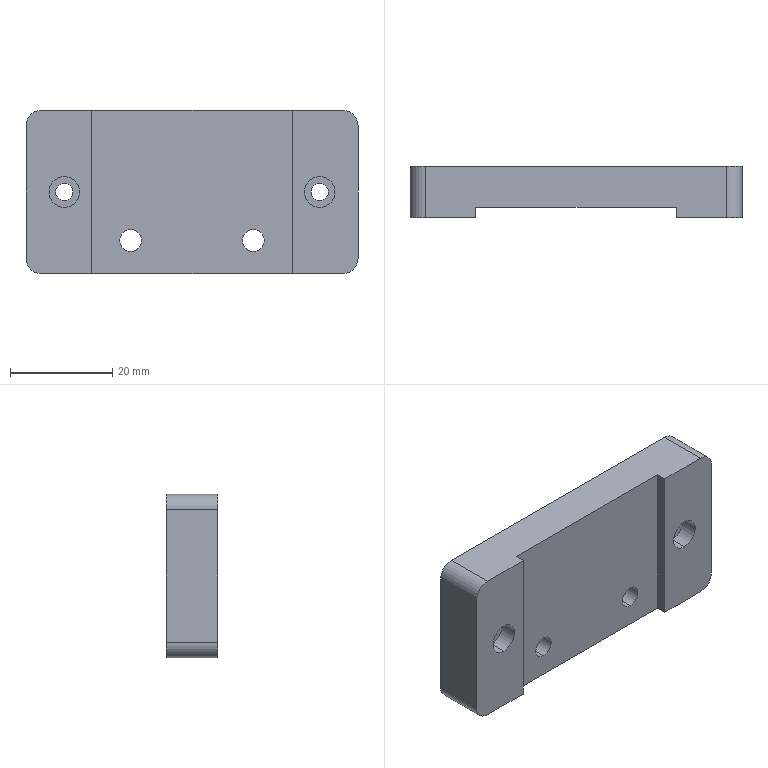Part | SolidWorks | features HoleWzd 3, ICE 3, Extrusion 1, Fillet 1 | 1 solid | 40 faces | box 65 x 10 x 32 mm | volume 16925 mm3 | cylinder 24 | plane 16 | commonest cylinder face diameters 6 x8 3.4 x4 4.3 x4 8 x4 12 x4
STEP:
#1=CARTESIAN_POINT('',(-12.,0.4,2.5));
#2=VERTEX_POINT('',#1);
#3=CARTESIAN_POINT('',(-12.,0.4,10.5));
#4=VERTEX_POINT('',#3);
#5=CARTESIAN_POINT('',(-12.,0.4,6.5));
#6=DIRECTION('',(0.,1.,0.));
#7=DIRECTION('',(0.,0.,1.));
#8=AXIS2_PLACEMENT_3D('',#5,#6,#7);
#9=CIRCLE('',#8,4.);
#10=EDGE_CURVE('',#2,#4,#9,.T.);
#11=ORIENTED_EDGE('',*,*,#10,.F.);
#12=CARTESIAN_POINT('',(-12.,5.,2.5));
#13=VERTEX_POINT('',#12);
#14=CARTESIAN_POINT('',(-12.,5.,2.5));
#15=DIRECTION('',(0.,1.,0.));
#16=VECTOR('',#15,1000.);
#17=LINE('',#14,#16);
#18=EDGE_CURVE('',#2,#13,#17,.T.);
#19=ORIENTED_EDGE('',*,*,#18,.T.);
#20=CARTESIAN_POINT('',(-12.,5.,10.5));
#21=VERTEX_POINT('',#20);
#22=CARTESIAN_POINT('',(-12.,5.,6.5));
#23=DIRECTION('',(0.,1.,0.));
#24=DIRECTION('',(0.,0.,1.));
#25=AXIS2_PLACEMENT_3D('',#22,#23,#24);
#26=CIRCLE('',#25,4.);
#27=EDGE_CURVE('',#13,#21,#26,.T.);
#28=ORIENTED_EDGE('',*,*,#27,.T.);
#29=CARTESIAN_POINT('',(-12.,5.,10.5));
#30=DIRECTION('',(0.,1.,0.));
#31=VECTOR('',#30,1000.);
#32=LINE('',#29,#31);
#33=EDGE_CURVE('',#4,#21,#32,.T.);
#34=ORIENTED_EDGE('',*,*,#33,.F.);
#35=EDGE_LOOP('',(#11,#19,#28,#34));
#36=FACE_OUTER_BOUND('',#35,.T.);
#37=CARTESIAN_POINT('',(-12.,5.,6.5));
#38=DIRECTION('',(0.,1.,0.));
#39=DIRECTION('',(0.,0.,1.));
#40=AXIS2_PLACEMENT_3D('',#37,#38,#39);
#41=CYLINDRICAL_SURFACE('',#40,4.);
#42=ADVANCED_FACE('',(#36),#41,.F.);
#43=CARTESIAN_POINT('',(12.,0.4,2.5));
#44=VERTEX_POINT('',#43);
#45=CARTESIAN_POINT('',(12.,0.4,10.5));
#46=VERTEX_POINT('',#45);
#47=CARTESIAN_POINT('',(12.,0.4,6.5));
#48=DIRECTION('',(0.,1.,0.));
#49=DIRECTION('',(0.,0.,1.));
#50=AXIS2_PLACEMENT_3D('',#47,#48,#49);
#51=CIRCLE('',#50,4.);
#52=EDGE_CURVE('',#44,#46,#51,.T.);
#53=ORIENTED_EDGE('',*,*,#52,.F.);
#54=CARTESIAN_POINT('',(12.,5.,2.5));
#55=VERTEX_POINT('',#54);
#56=CARTESIAN_POINT('',(12.,5.,2.5));
#57=DIRECTION('',(0.,1.,0.));
#58=VECTOR('',#57,1000.);
#59=LINE('',#56,#58);
#60=EDGE_CURVE('',#44,#55,#59,.T.);
#61=ORIENTED_EDGE('',*,*,#60,.T.);
#62=CARTESIAN_POINT('',(12.,5.,10.5));
#63=VERTEX_POINT('',#62);
#64=CARTESIAN_POINT('',(12.,5.,6.5));
#65=DIRECTION('',(0.,1.,0.));
#66=DIRECTION('',(0.,0.,1.));
#67=AXIS2_PLACEMENT_3D('',#64,#65,#66);
#68=CIRCLE('',#67,4.);
#69=EDGE_CURVE('',#55,#63,#68,.T.);
#70=ORIENTED_EDGE('',*,*,#69,.T.);
#71=CARTESIAN_POINT('',(12.,5.,10.5));
#72=DIRECTION('',(0.,1.,0.));
#73=VECTOR('',#72,1000.);
#74=LINE('',#71,#73);
#75=EDGE_CURVE('',#46,#63,#74,.T.);
#76=ORIENTED_EDGE('',*,*,#75,.F.);
#77=EDGE_LOOP('',(#53,#61,#70,#76));
#78=FACE_OUTER_BOUND('',#77,.T.);
#79=CARTESIAN_POINT('',(12.,5.,6.5));
#80=DIRECTION('',(0.,1.,0.));
#81=DIRECTION('',(0.,0.,1.));
#82=AXIS2_PLACEMENT_3D('',#79,#80,#81);
#83=CYLINDRICAL_SURFACE('',#82,4.);
#84=ADVANCED_FACE('',(#78),#83,.F.);
#85=CARTESIAN_POINT('',(25.,-1.6,19.));
#86=VERTEX_POINT('',#85);
#87=CARTESIAN_POINT('',(25.,-1.6,13.));
#88=VERTEX_POINT('',#87);
#89=CARTESIAN_POINT('',(25.,-1.6,16.));
#90=DIRECTION('',(0.,-1.,0.));
#91=DIRECTION('',(0.,0.,-1.));
#92=AXIS2_PLACEMENT_3D('',#89,#90,#91);
#93=CIRCLE('',#92,3.);
#94=EDGE_CURVE('',#86,#88,#93,.T.);
#95=ORIENTED_EDGE('',*,*,#94,.F.);
#96=CARTESIAN_POINT('',(25.,-5.,19.));
#97=VERTEX_POINT('',#96);
#98=CARTESIAN_POINT('',(25.,-5.,19.));
#99=DIRECTION('',(0.,-1.,0.));
#100=VECTOR('',#99,1000.);
#101=LINE('',#98,#100);
#102=EDGE_CURVE('',#86,#97,#101,.T.);
#103=ORIENTED_EDGE('',*,*,#102,.T.);
#104=CARTESIAN_POINT('',(25.,-5.,13.));
#105=VERTEX_POINT('',#104);
#106=CARTESIAN_POINT('',(25.,-5.,16.));
#107=DIRECTION('',(0.,-1.,0.));
#108=DIRECTION('',(0.,0.,-1.));
#109=AXIS2_PLACEMENT_3D('',#106,#107,#108);
#110=CIRCLE('',#109,3.);
#111=EDGE_CURVE('',#97,#105,#110,.T.);
#112=ORIENTED_EDGE('',*,*,#111,.T.);
#113=CARTESIAN_POINT('',(25.,-5.,13.));
#114=DIRECTION('',(0.,-1.,0.));
#115=VECTOR('',#114,1000.);
#116=LINE('',#113,#115);
#117=EDGE_CURVE('',#88,#105,#116,.T.);
#118=ORIENTED_EDGE('',*,*,#117,.F.);
#119=EDGE_LOOP('',(#95,#103,#112,#118));
#120=FACE_OUTER_BOUND('',#119,.T.);
#121=CARTESIAN_POINT('',(25.,-5.,16.));
#122=DIRECTION('',(0.,-1.,0.));
#123=DIRECTION('',(0.,0.,-1.));
#124=AXIS2_PLACEMENT_3D('',#121,#122,#123);
#125=CYLINDRICAL_SURFACE('',#124,3.);
#126=ADVANCED_FACE('',(#120),#125,.F.);
#127=CARTESIAN_POINT('',(25.,3.,17.7));
#128=VERTEX_POINT('',#127);
#129=CARTESIAN_POINT('',(25.,3.,14.3));
#130=VERTEX_POINT('',#129);
#131=CARTESIAN_POINT('',(25.,3.,16.));
#132=DIRECTION('',(0.,-1.,0.));
#133=DIRECTION('',(0.,0.,-1.));
#134=AXIS2_PLACEMENT_3D('',#131,#132,#133);
#135=CIRCLE('',#134,1.7);
#136=EDGE_CURVE('',#128,#130,#135,.T.);
#137=ORIENTED_EDGE('',*,*,#136,.F.);
#138=CARTESIAN_POINT('',(25.,-1.6,17.7));
#139=VERTEX_POINT('',#138);
#140=CARTESIAN_POINT('',(25.,-5.,17.7));
#141=DIRECTION('',(0.,-1.,0.));
#142=VECTOR('',#141,1000.);
#143=LINE('',#140,#142);
#144=EDGE_CURVE('',#128,#139,#143,.T.);
#145=ORIENTED_EDGE('',*,*,#144,.T.);
#146=CARTESIAN_POINT('',(25.,-1.6,14.3));
#147=VERTEX_POINT('',#146);
#148=CARTESIAN_POINT('',(25.,-1.6,16.));
#149=DIRECTION('',(0.,-1.,0.));
#150=DIRECTION('',(0.,0.,-1.));
#151=AXIS2_PLACEMENT_3D('',#148,#149,#150);
#152=CIRCLE('',#151,1.7);
#153=EDGE_CURVE('',#139,#147,#152,.T.);
#154=ORIENTED_EDGE('',*,*,#153,.T.);
#155=CARTESIAN_POINT('',(25.,-5.,14.3));
#156=DIRECTION('',(0.,-1.,0.));
#157=VECTOR('',#156,1000.);
#158=LINE('',#155,#157);
#159=EDGE_CURVE('',#130,#147,#158,.T.);
#160=ORIENTED_EDGE('',*,*,#159,.F.);
#161=EDGE_LOOP('',(#137,#145,#154,#160));
#162=FACE_OUTER_BOUND('',#161,.T.);
#163=CARTESIAN_POINT('',(25.,-5.,16.));
#164=DIRECTION('',(0.,-1.,0.));
#165=DIRECTION('',(0.,0.,-1.));
#166=AXIS2_PLACEMENT_3D('',#163,#164,#165);
#167=CYLINDRICAL_SURFACE('',#166,1.7);
#168=ADVANCED_FACE('',(#162),#167,.F.);
#169=CARTESIAN_POINT('',(-25.,-1.6,19.));
#170=VERTEX_POINT('',#169);
#171=CARTESIAN_POINT('',(-25.,-1.6,13.));
#172=VERTEX_POINT('',#171);
#173=CARTESIAN_POINT('',(-25.,-1.6,16.));
#174=DIRECTION('',(0.,-1.,0.));
#175=DIRECTION('',(0.,0.,-1.));
#176=AXIS2_PLACEMENT_3D('',#173,#174,#175);
#177=CIRCLE('',#176,3.);
#178=EDGE_CURVE('',#170,#172,#177,.T.);
#179=ORIENTED_EDGE('',*,*,#178,.F.);
#180=CARTESIAN_POINT('',(-25.,-5.,19.));
#181=VERTEX_POINT('',#180);
#182=CARTESIAN_POINT('',(-25.,-5.,19.));
#183=DIRECTION('',(0.,-1.,0.));
#184=VECTOR('',#183,1000.);
#185=LINE('',#182,#184);
#186=EDGE_CURVE('',#170,#181,#185,.T.);
#187=ORIENTED_EDGE('',*,*,#186,.T.);
#188=CARTESIAN_POINT('',(-25.,-5.,13.));
#189=VERTEX_POINT('',#188);
#190=CARTESIAN_POINT('',(-25.,-5.,16.));
#191=DIRECTION('',(0.,-1.,0.));
#192=DIRECTION('',(0.,0.,-1.));
#193=AXIS2_PLACEMENT_3D('',#190,#191,#192);
#194=CIRCLE('',#193,3.);
#195=EDGE_CURVE('',#181,#189,#194,.T.);
#196=ORIENTED_EDGE('',*,*,#195,.T.);
#197=CARTESIAN_POINT('',(-25.,-5.,13.));
#198=DIRECTION('',(0.,-1.,0.));
#199=VECTOR('',#198,1000.);
#200=LINE('',#197,#199);
#201=EDGE_CURVE('',#172,#189,#200,.T.);
#202=ORIENTED_EDGE('',*,*,#201,.F.);
#203=EDGE_LOOP('',(#179,#187,#196,#202));
#204=FACE_OUTER_BOUND('',#203,.T.);
#205=CARTESIAN_POINT('',(-25.,-5.,16.));
#206=DIRECTION('',(0.,-1.,0.));
#207=DIRECTION('',(0.,0.,-1.));
#208=AXIS2_PLACEMENT_3D('',#205,#206,#207);
#209=CYLINDRICAL_SURFACE('',#208,3.);
#210=ADVANCED_FACE('',(#204),#209,.F.);
#211=CARTESIAN_POINT('',(-25.,3.,14.3));
#212=VERTEX_POINT('',#211);
#213=CARTESIAN_POINT('',(-25.,3.,17.7));
#214=VERTEX_POINT('',#213);
#215=CARTESIAN_POINT('',(-25.,3.,16.));
#216=DIRECTION('',(0.,1.,0.));
#217=DIRECTION('',(0.,0.,1.));
#218=AXIS2_PLACEMENT_3D('',#215,#216,#217);
#219=CIRCLE('',#218,1.7);
#220=EDGE_CURVE('',#212,#214,#219,.T.);
#221=ORIENTED_EDGE('',*,*,#220,.T.);
#222=CARTESIAN_POINT('',(-25.,-1.6,17.7));
#223=VERTEX_POINT('',#222);
#224=CARTESIAN_POINT('',(-25.,-5.,17.7));
#225=DIRECTION('',(0.,-1.,0.));
#226=VECTOR('',#225,1000.);
#227=LINE('',#224,#226);
#228=EDGE_CURVE('',#214,#223,#227,.T.);
#229=ORIENTED_EDGE('',*,*,#228,.T.);
#230=CARTESIAN_POINT('',(-25.,-1.6,14.3));
#231=VERTEX_POINT('',#230);
#232=CARTESIAN_POINT('',(-25.,-1.6,16.));
#233=DIRECTION('',(0.,-1.,0.));
#234=DIRECTION('',(0.,0.,-1.));
#235=AXIS2_PLACEMENT_3D('',#232,#233,#234);
#236=CIRCLE('',#235,1.7);
#237=EDGE_CURVE('',#223,#231,#236,.T.);
#238=ORIENTED_EDGE('',*,*,#237,.T.);
#239=CARTESIAN_POINT('',(-25.,-5.,14.3));
#240=DIRECTION('',(0.,-1.,0.));
#241=VECTOR('',#240,1000.);
#242=LINE('',#239,#241);
#243=EDGE_CURVE('',#212,#231,#242,.T.);
#244=ORIENTED_EDGE('',*,*,#243,.F.);
#245=EDGE_LOOP('',(#221,#229,#238,#244));
#246=FACE_OUTER_BOUND('',#245,.T.);
#247=CARTESIAN_POINT('',(-25.,-5.,16.));
#248=DIRECTION('',(0.,-1.,0.));
#249=DIRECTION('',(0.,0.,-1.));
#250=AXIS2_PLACEMENT_3D('',#247,#248,#249);
#251=CYLINDRICAL_SURFACE('',#250,1.7);
#252=ADVANCED_FACE('',(#246),#251,.F.);
#253=CARTESIAN_POINT('',(25.,3.,10.));
#254=VERTEX_POINT('',#253);
#255=CARTESIAN_POINT('',(25.,3.,22.));
#256=VERTEX_POINT('',#255);
#257=CARTESIAN_POINT('',(25.,3.,16.));
#258=DIRECTION('',(0.,1.,0.));
#259=DIRECTION('',(0.,0.,-1.));
#260=AXIS2_PLACEMENT_3D('',#257,#258,#259);
#261=CIRCLE('',#260,6.);
#262=EDGE_CURVE('',#254,#256,#261,.T.);
#263=ORIENTED_EDGE('',*,*,#262,.F.);
#264=CARTESIAN_POINT('',(25.,5.,10.));
#265=VERTEX_POINT('',#264);
#266=CARTESIAN_POINT('',(25.,3.,10.));
#267=DIRECTION('',(0.,1.,0.));
#268=VECTOR('',#267,1000.);
#269=LINE('',#266,#268);
#270=EDGE_CURVE('',#254,#265,#269,.T.);
#271=ORIENTED_EDGE('',*,*,#270,.T.);
#272=CARTESIAN_POINT('',(25.,5.,22.));
#273=VERTEX_POINT('',#272);
#274=CARTESIAN_POINT('',(25.,5.,16.));
#275=DIRECTION('',(0.,1.,0.));
#276=DIRECTION('',(0.,0.,-1.));
#277=AXIS2_PLACEMENT_3D('',#274,#275,#276);
#278=CIRCLE('',#277,6.);
#279=EDGE_CURVE('',#265,#273,#278,.T.);
#280=ORIENTED_EDGE('',*,*,#279,.T.);
#281=CARTESIAN_POINT('',(25.,3.,22.));
#282=DIRECTION('',(0.,1.,0.));
#283=VECTOR('',#282,1000.);
#284=LINE('',#281,#283);
#285=EDGE_CURVE('',#256,#273,#284,.T.);
#286=ORIENTED_EDGE('',*,*,#285,.F.);
#287=EDGE_LOOP('',(#263,#271,#280,#286));
#288=FACE_OUTER_BOUND('',#287,.T.);
#289=CARTESIAN_POINT('',(25.,3.,16.));
#290=DIRECTION('',(0.,1.,0.));
#291=DIRECTION('',(0.,0.,1.));
#292=AXIS2_PLACEMENT_3D('',#289,#290,#291);
#293=CYLINDRICAL_SURFACE('',#292,6.);
#294=ADVANCED_FACE('',(#288),#293,.F.);
#295=CARTESIAN_POINT('',(-25.,3.,10.));
#296=VERTEX_POINT('',#295);
#297=CARTESIAN_POINT('',(-25.,3.,22.));
#298=VERTEX_POINT('',#297);
#299=CARTESIAN_POINT('',(-25.,3.,16.));
#300=DIRECTION('',(0.,1.,0.));
#301=DIRECTION('',(0.,0.,1.));
#302=AXIS2_PLACEMENT_3D('',#299,#300,#301);
#303=CIRCLE('',#302,6.);
#304=EDGE_CURVE('',#296,#298,#303,.T.);
#305=ORIENTED_EDGE('',*,*,#304,.F.);
#306=CARTESIAN_POINT('',(-25.,5.,10.));
#307=VERTEX_POINT('',#306);
#308=CARTESIAN_POINT('',(-25.,3.,10.));
#309=DIRECTION('',(0.,1.,0.));
#310=VECTOR('',#309,1000.);
#311=LINE('',#308,#310);
#312=EDGE_CURVE('',#296,#307,#311,.T.);
#313=ORIENTED_EDGE('',*,*,#312,.T.);
#314=CARTESIAN_POINT('',(-25.,5.,22.));
#315=VERTEX_POINT('',#314);
#316=CARTESIAN_POINT('',(-25.,5.,16.));
#317=DIRECTION('',(0.,1.,0.));
#318=DIRECTION('',(0.,0.,1.));
#319=AXIS2_PLACEMENT_3D('',#316,#317,#318);
#320=CIRCLE('',#319,6.);
#321=EDGE_CURVE('',#307,#315,#320,.T.);
#322=ORIENTED_EDGE('',*,*,#321,.T.);
#323=CARTESIAN_POINT('',(-25.,3.,22.));
#324=DIRECTION('',(0.,1.,0.));
#325=VECTOR('',#324,1000.);
#326=LINE('',#323,#325);
#327=EDGE_CURVE('',#298,#315,#326,.T.);
#328=ORIENTED_EDGE('',*,*,#327,.F.);
#329=EDGE_LOOP('',(#305,#313,#322,#328));
#330=FACE_OUTER_BOUND('',#329,.T.);
#331=CARTESIAN_POINT('',(-25.,3.,16.));
#332=DIRECTION('',(0.,1.,0.));
#333=DIRECTION('',(0.,0.,1.));
#334=AXIS2_PLACEMENT_3D('',#331,#332,#333);
#335=CYLINDRICAL_SURFACE('',#334,6.);
#336=ADVANCED_FACE('',(#330),#335,.F.);
#337=CARTESIAN_POINT('',(-12.,0.4,4.35));
#338=VERTEX_POINT('',#337);
#339=CARTESIAN_POINT('',(-12.,0.4,8.65));
#340=VERTEX_POINT('',#339);
#341=CARTESIAN_POINT('',(-12.,0.4,6.5));
#342=DIRECTION('',(0.,1.,0.));
#343=DIRECTION('',(0.,0.,1.));
#344=AXIS2_PLACEMENT_3D('',#341,#342,#343);
#345=CIRCLE('',#344,2.15);
#346=EDGE_CURVE('',#338,#340,#345,.T.);
#347=ORIENTED_EDGE('',*,*,#346,.T.);
#348=CARTESIAN_POINT('',(-12.,-3.,8.65));
#349=VERTEX_POINT('',#348);
#350=CARTESIAN_POINT('',(-12.,-5.,8.65));
#351=DIRECTION('',(0.,-1.,0.));
#352=VECTOR('',#351,1000.);
#353=LINE('',#350,#352);
#354=EDGE_CURVE('',#340,#349,#353,.T.);
#355=ORIENTED_EDGE('',*,*,#354,.T.);
#356=CARTESIAN_POINT('',(-12.,-3.,4.35));
#357=VERTEX_POINT('',#356);
#358=CARTESIAN_POINT('',(-12.,-3.,6.5));
#359=DIRECTION('',(0.,-1.,0.));
#360=DIRECTION('',(0.,0.,1.));
#361=AXIS2_PLACEMENT_3D('',#358,#359,#360);
#362=CIRCLE('',#361,2.15);
#363=EDGE_CURVE('',#349,#357,#362,.T.);
#364=ORIENTED_EDGE('',*,*,#363,.T.);
#365=CARTESIAN_POINT('',(-12.,-5.,4.35));
#366=DIRECTION('',(0.,-1.,0.));
#367=VECTOR('',#366,1000.);
#368=LINE('',#365,#367);
#369=EDGE_CURVE('',#338,#357,#368,.T.);
#370=ORIENTED_EDGE('',*,*,#369,.F.);
#371=EDGE_LOOP('',(#347,#355,#364,#370));
#372=FACE_OUTER_BOUND('',#371,.T.);
#373=CARTESIAN_POINT('',(-12.,-5.,6.5));
#374=DIRECTION('',(0.,-1.,0.));
#375=DIRECTION('',(0.,0.,-1.));
#376=AXIS2_PLACEMENT_3D('',#373,#374,#375);
#377=CYLINDRICAL_SURFACE('',#376,2.15);
#378=ADVANCED_FACE('',(#372),#377,.F.);
#379=CARTESIAN_POINT('',(12.,0.4,4.35));
#380=VERTEX_POINT('',#379);
#381=CARTESIAN_POINT('',(12.,0.4,8.65));
#382=VERTEX_POINT('',#381);
#383=CARTESIAN_POINT('',(12.,0.4,6.5));
#384=DIRECTION('',(0.,1.,0.));
#385=DIRECTION('',(0.,0.,1.));
#386=AXIS2_PLACEMENT_3D('',#383,#384,#385);
#387=CIRCLE('',#386,2.15);
#388=EDGE_CURVE('',#380,#382,#387,.T.);
#389=ORIENTED_EDGE('',*,*,#388,.T.);
#390=CARTESIAN_POINT('',(12.,-3.,8.65));
#391=VERTEX_POINT('',#390);
#392=CARTESIAN_POINT('',(12.,-5.,8.65));
#393=DIRECTION('',(0.,-1.,0.));
#394=VECTOR('',#393,1000.);
#395=LINE('',#392,#394);
#396=EDGE_CURVE('',#382,#391,#395,.T.);
#397=ORIENTED_EDGE('',*,*,#396,.T.);
#398=CARTESIAN_POINT('',(12.,-3.,4.35));
#399=VERTEX_POINT('',#398);
#400=CARTESIAN_POINT('',(12.,-3.,6.5));
#401=DIRECTION('',(0.,-1.,0.));
#402=DIRECTION('',(0.,0.,1.));
#403=AXIS2_PLACEMENT_3D('',#400,#401,#402);
#404=CIRCLE('',#403,2.15);
#405=EDGE_CURVE('',#391,#399,#404,.T.);
#406=ORIENTED_EDGE('',*,*,#405,.T.);
#407=CARTESIAN_POINT('',(12.,-5.,4.35));
#408=DIRECTION('',(0.,-1.,0.));
#409=VECTOR('',#408,1000.);
#410=LINE('',#407,#409);
#411=EDGE_CURVE('',#380,#399,#410,.T.);
#412=ORIENTED_EDGE('',*,*,#411,.F.);
#413=EDGE_LOOP('',(#389,#397,#406,#412));
#414=FACE_OUTER_BOUND('',#413,.T.);
#415=CARTESIAN_POINT('',(12.,-5.,6.5));
#416=DIRECTION('',(0.,-1.,0.));
#417=DIRECTION('',(0.,0.,-1.));
#418=AXIS2_PLACEMENT_3D('',#415,#416,#417);
#419=CYLINDRICAL_SURFACE('',#418,2.15);
#420=ADVANCED_FACE('',(#414),#419,.F.);
#421=CARTESIAN_POINT('',(25.,-5.,16.));
#422=DIRECTION('',(0.,-1.,0.));
#423=DIRECTION('',(0.,0.,-1.));
#424=AXIS2_PLACEMENT_3D('',#421,#422,#423);
#425=CIRCLE('',#424,3.);
#426=EDGE_CURVE('',#105,#97,#425,.T.);
#427=ORIENTED_EDGE('',*,*,#426,.F.);
#428=ORIENTED_EDGE('',*,*,#111,.F.);
#429=EDGE_LOOP('',(#427,#428));
#430=FACE_BOUND('',#429,.T.);
#431=CARTESIAN_POINT('',(19.6,-5.,32.));
#432=VERTEX_POINT('',#431);
#433=CARTESIAN_POINT('',(29.5,-5.,32.));
#434=VERTEX_POINT('',#433);
#435=CARTESIAN_POINT('',(-32.5,-5.,32.));
#436=DIRECTION('',(1.,0.,0.));
#437=VECTOR('',#436,1000.);
#438=LINE('',#435,#437);
#439=EDGE_CURVE('',#432,#434,#438,.T.);
#440=ORIENTED_EDGE('',*,*,#439,.F.);
#441=CARTESIAN_POINT('',(19.6,-5.,0.));
#442=VERTEX_POINT('',#441);
#443=CARTESIAN_POINT('',(19.6,-5.,-36.442));
#444=DIRECTION('',(0.,0.,1.));
#445=VECTOR('',#444,1000.);
#446=LINE('',#443,#445);
#447=EDGE_CURVE('',#442,#432,#446,.T.);
#448=ORIENTED_EDGE('',*,*,#447,.F.);
#449=CARTESIAN_POINT('',(29.5,-5.,0.));
#450=VERTEX_POINT('',#449);
#451=CARTESIAN_POINT('',(-32.5,-5.,0.));
#452=DIRECTION('',(1.,0.,0.));
#453=VECTOR('',#452,1000.);
#454=LINE('',#451,#453);
#455=EDGE_CURVE('',#442,#450,#454,.T.);
#456=ORIENTED_EDGE('',*,*,#455,.T.);
#457=CARTESIAN_POINT('',(32.5,-5.,3.));
#458=VERTEX_POINT('',#457);
#459=CARTESIAN_POINT('',(29.5,-5.,3.));
#460=DIRECTION('',(0.,-1.,0.));
#461=DIRECTION('',(0.,0.,1.));
#462=AXIS2_PLACEMENT_3D('',#459,#460,#461);
#463=CIRCLE('',#462,3.);
#464=EDGE_CURVE('',#450,#458,#463,.T.);
#465=ORIENTED_EDGE('',*,*,#464,.T.);
#466=CARTESIAN_POINT('',(32.5,-5.,29.));
#467=VERTEX_POINT('',#466);
#468=CARTESIAN_POINT('',(32.5,-5.,32.));
#469=DIRECTION('',(0.,0.,-1.));
#470=VECTOR('',#469,1000.);
#471=LINE('',#468,#470);
#472=EDGE_CURVE('',#467,#458,#471,.T.);
#473=ORIENTED_EDGE('',*,*,#472,.F.);
#474=CARTESIAN_POINT('',(29.5,-5.,29.));
#475=DIRECTION('',(0.,-1.,0.));
#476=DIRECTION('',(0.,0.,1.));
#477=AXIS2_PLACEMENT_3D('',#474,#475,#476);
#478=CIRCLE('',#477,3.);
#479=EDGE_CURVE('',#467,#434,#478,.T.);
#480=ORIENTED_EDGE('',*,*,#479,.T.);
#481=EDGE_LOOP('',(#440,#448,#456,#465,#473,#480));
#482=FACE_OUTER_BOUND('',#481,.T.);
#483=CARTESIAN_POINT('',(-32.5,-5.,32.));
#484=DIRECTION('',(0.,1.,0.));
#485=DIRECTION('',(0.,0.,1.));
#486=AXIS2_PLACEMENT_3D('',#483,#484,#485);
#487=PLANE('',#486);
#488=ADVANCED_FACE('',(#430,#482),#487,.F.);
#489=CARTESIAN_POINT('',(-12.,5.,6.5));
#490=DIRECTION('',(0.,1.,0.));
#491=DIRECTION('',(0.,0.,1.));
#492=AXIS2_PLACEMENT_3D('',#489,#490,#491);
#493=CIRCLE('',#492,4.);
#494=EDGE_CURVE('',#21,#13,#493,.T.);
#495=ORIENTED_EDGE('',*,*,#494,.F.);
#496=ORIENTED_EDGE('',*,*,#27,.F.);
#497=EDGE_LOOP('',(#495,#496));
#498=FACE_BOUND('',#497,.T.);
#499=CARTESIAN_POINT('',(29.5,5.,0.));
#500=VERTEX_POINT('',#499);
#501=CARTESIAN_POINT('',(-29.5,5.,0.));
#502=VERTEX_POINT('',#501);
#503=CARTESIAN_POINT('',(-32.5,5.,0.));
#504=DIRECTION('',(-1.,0.,0.));
#505=VECTOR('',#504,1000.);
#506=LINE('',#503,#505);
#507=EDGE_CURVE('',#500,#502,#506,.T.);
#508=ORIENTED_EDGE('',*,*,#507,.T.);
#509=CARTESIAN_POINT('',(-32.5,5.,3.));
#510=VERTEX_POINT('',#509);
#511=CARTESIAN_POINT('',(-29.5,5.,3.));
#512=DIRECTION('',(0.,1.,0.));
#513=DIRECTION('',(0.,0.,-1.));
#514=AXIS2_PLACEMENT_3D('',#511,#512,#513);
#515=CIRCLE('',#514,3.);
#516=EDGE_CURVE('',#502,#510,#515,.T.);
#517=ORIENTED_EDGE('',*,*,#516,.T.);
#518=CARTESIAN_POINT('',(-32.5,5.,29.));
#519=VERTEX_POINT('',#518);
#520=CARTESIAN_POINT('',(-32.5,5.,32.));
#521=DIRECTION('',(0.,0.,-1.));
#522=VECTOR('',#521,1000.);
#523=LINE('',#520,#522);
#524=EDGE_CURVE('',#519,#510,#523,.T.);
#525=ORIENTED_EDGE('',*,*,#524,.F.);
#526=CARTESIAN_POINT('',(-29.5,5.,32.));
#527=VERTEX_POINT('',#526);
#528=CARTESIAN_POINT('',(-29.5,5.,29.));
#529=DIRECTION('',(0.,1.,0.));
#530=DIRECTION('',(0.,0.,-1.));
#531=AXIS2_PLACEMENT_3D('',#528,#529,#530);
#532=CIRCLE('',#531,3.);
#533=EDGE_CURVE('',#519,#527,#532,.T.);
#534=ORIENTED_EDGE('',*,*,#533,.T.);
#535=CARTESIAN_POINT('',(29.5,5.,32.));
#536=VERTEX_POINT('',#535);
#537=CARTESIAN_POINT('',(-32.5,5.,32.));
#538=DIRECTION('',(-1.,0.,0.));
#539=VECTOR('',#538,1000.);
#540=LINE('',#537,#539);
#541=EDGE_CURVE('',#536,#527,#540,.T.);
#542=ORIENTED_EDGE('',*,*,#541,.F.);
#543=CARTESIAN_POINT('',(32.5,5.,29.));
#544=VERTEX_POINT('',#543);
#545=CARTESIAN_POINT('',(29.5,5.,29.));
#546=DIRECTION('',(0.,1.,0.));
#547=DIRECTION('',(0.,0.,-1.));
#548=AXIS2_PLACEMENT_3D('',#545,#546,#547);
#549=CIRCLE('',#548,3.);
#550=EDGE_CURVE('',#536,#544,#549,.T.);
#551=ORIENTED_EDGE('',*,*,#550,.T.);
#552=CARTESIAN_POINT('',(32.5,5.,3.));
#553=VERTEX_POINT('',#552);
#554=CARTESIAN_POINT('',(32.5,5.,32.));
#555=DIRECTION('',(0.,0.,-1.));
#556=VECTOR('',#555,1000.);
#557=LINE('',#554,#556);
#558=EDGE_CURVE('',#544,#553,#557,.T.);
#559=ORIENTED_EDGE('',*,*,#558,.T.);
#560=CARTESIAN_POINT('',(29.5,5.,3.));
#561=DIRECTION('',(0.,1.,0.));
#562=DIRECTION('',(0.,0.,-1.));
#563=AXIS2_PLACEMENT_3D('',#560,#561,#562);
#564=CIRCLE('',#563,3.);
#565=EDGE_CURVE('',#553,#500,#564,.T.);
#566=ORIENTED_EDGE('',*,*,#565,.T.);
#567=EDGE_LOOP('',(#508,#517,#525,#534,#542,#551,#559,#566));
#568=FACE_OUTER_BOUND('',#567,.T.);
#569=CARTESIAN_POINT('',(-25.,5.,16.));
#570=DIRECTION('',(0.,1.,0.));
#571=DIRECTION('',(0.,0.,1.));
#572=AXIS2_PLACEMENT_3D('',#569,#570,#571);
#573=CIRCLE('',#572,6.);
#574=EDGE_CURVE('',#315,#307,#573,.T.);
#575=ORIENTED_EDGE('',*,*,#574,.F.);
#576=ORIENTED_EDGE('',*,*,#321,.F.);
#577=EDGE_LOOP('',(#575,#576));
#578=FACE_BOUND('',#577,.T.);
#579=CARTESIAN_POINT('',(25.,5.,16.));
#580=DIRECTION('',(0.,1.,0.));
#581=DIRECTION('',(0.,0.,-1.));
#582=AXIS2_PLACEMENT_3D('',#579,#580,#581);
#583=CIRCLE('',#582,6.);
#584=EDGE_CURVE('',#273,#265,#583,.T.);
#585=ORIENTED_EDGE('',*,*,#584,.F.);
#586=ORIENTED_EDGE('',*,*,#279,.F.);
#587=EDGE_LOOP('',(#585,#586));
#588=FACE_BOUND('',#587,.T.);
#589=CARTESIAN_POINT('',(12.,5.,6.5));
#590=DIRECTION('',(0.,1.,0.));
#591=DIRECTION('',(0.,0.,1.));
#592=AXIS2_PLACEMENT_3D('',#589,#590,#591);
#593=CIRCLE('',#592,4.);
#594=EDGE_CURVE('',#63,#55,#593,.T.);
#595=ORIENTED_EDGE('',*,*,#594,.F.);
#596=ORIENTED_EDGE('',*,*,#69,.F.);
#597=EDGE_LOOP('',(#595,#596));
#598=FACE_BOUND('',#597,.T.);
#599=CARTESIAN_POINT('',(-32.5,5.,32.));
#600=DIRECTION('',(0.,-1.,0.));
#601=DIRECTION('',(0.,0.,-1.));
#602=AXIS2_PLACEMENT_3D('',#599,#600,#601);
#603=PLANE('',#602);
#604=ADVANCED_FACE('',(#498,#568,#578,#588,#598),#603,.F.);
#605=ORIENTED_EDGE('',*,*,#472,.T.);
#606=CARTESIAN_POINT('',(32.5,5.,3.));
#607=DIRECTION('',(0.,1.,0.));
#608=VECTOR('',#607,1000.);
#609=LINE('',#606,#608);
#610=EDGE_CURVE('',#458,#553,#609,.T.);
#611=ORIENTED_EDGE('',*,*,#610,.T.);
#612=ORIENTED_EDGE('',*,*,#558,.F.);
#613=CARTESIAN_POINT('',(32.5,-5.,29.));
#614=DIRECTION('',(0.,-1.,0.));
#615=VECTOR('',#614,1000.);
#616=LINE('',#613,#615);
#617=EDGE_CURVE('',#544,#467,#616,.T.);
#618=ORIENTED_EDGE('',*,*,#617,.T.);
#619=EDGE_LOOP('',(#605,#611,#612,#618));
#620=FACE_OUTER_BOUND('',#619,.T.);
#621=CARTESIAN_POINT('',(32.5,5.,32.));
#622=DIRECTION('',(-1.,0.,0.));
#623=DIRECTION('',(0.,0.,1.));
#624=AXIS2_PLACEMENT_3D('',#621,#622,#623);
#625=PLANE('',#624);
#626=ADVANCED_FACE('',(#620),#625,.F.);
#627=ORIENTED_EDGE('',*,*,#524,.T.);
#628=CARTESIAN_POINT('',(-32.5,-5.,3.));
#629=VERTEX_POINT('',#628);
#630=CARTESIAN_POINT('',(-32.5,5.,3.));
#631=DIRECTION('',(0.,-1.,0.));
#632=VECTOR('',#631,1000.);
#633=LINE('',#630,#632);
#634=EDGE_CURVE('',#510,#629,#633,.T.);
#635=ORIENTED_EDGE('',*,*,#634,.T.);
#636=CARTESIAN_POINT('',(-32.5,-5.,29.));
#637=VERTEX_POINT('',#636);
#638=CARTESIAN_POINT('',(-32.5,-5.,32.));
#639=DIRECTION('',(0.,0.,-1.));
#640=VECTOR('',#639,1000.);
#641=LINE('',#638,#640);
#642=EDGE_CURVE('',#637,#629,#641,.T.);
#643=ORIENTED_EDGE('',*,*,#642,.F.);
#644=CARTESIAN_POINT('',(-32.5,5.,29.));
#645=DIRECTION('',(0.,1.,0.));
#646=VECTOR('',#645,1000.);
#647=LINE('',#644,#646);
#648=EDGE_CURVE('',#637,#519,#647,.T.);
#649=ORIENTED_EDGE('',*,*,#648,.T.);
#650=EDGE_LOOP('',(#627,#635,#643,#649));
#651=FACE_OUTER_BOUND('',#650,.T.);
#652=CARTESIAN_POINT('',(-32.5,5.,32.));
#653=DIRECTION('',(1.,0.,0.));
#654=DIRECTION('',(0.,0.,-1.));
#655=AXIS2_PLACEMENT_3D('',#652,#653,#654);
#656=PLANE('',#655);
#657=ADVANCED_FACE('',(#651),#656,.F.);
#658=CARTESIAN_POINT('',(-25.,-5.,16.));
#659=DIRECTION('',(0.,-1.,0.));
#660=DIRECTION('',(0.,0.,-1.));
#661=AXIS2_PLACEMENT_3D('',#658,#659,#660);
#662=CIRCLE('',#661,3.);
#663=EDGE_CURVE('',#189,#181,#662,.T.);
#664=ORIENTED_EDGE('',*,*,#663,.F.);
#665=ORIENTED_EDGE('',*,*,#195,.F.);
#666=EDGE_LOOP('',(#664,#665));
#667=FACE_BOUND('',#666,.T.);
#668=CARTESIAN_POINT('',(-29.5,-5.,0.));
#669=VERTEX_POINT('',#668);
#670=CARTESIAN_POINT('',(-19.6,-5.,0.));
#671=VERTEX_POINT('',#670);
#672=CARTESIAN_POINT('',(-32.5,-5.,0.));
#673=DIRECTION('',(1.,0.,0.));
#674=VECTOR('',#673,1000.);
#675=LINE('',#672,#674);
#676=EDGE_CURVE('',#669,#671,#675,.T.);
#677=ORIENTED_EDGE('',*,*,#676,.T.);
#678=CARTESIAN_POINT('',(-19.6,-5.,32.));
#679=VERTEX_POINT('',#678);
#680=CARTESIAN_POINT('',(-19.6,-5.,-36.442));
#681=DIRECTION('',(0.,0.,-1.));
#682=VECTOR('',#681,1000.);
#683=LINE('',#680,#682);
#684=EDGE_CURVE('',#679,#671,#683,.T.);
#685=ORIENTED_EDGE('',*,*,#684,.F.);
#686=CARTESIAN_POINT('',(-29.5,-5.,32.));
#687=VERTEX_POINT('',#686);
#688=CARTESIAN_POINT('',(-32.5,-5.,32.));
#689=DIRECTION('',(1.,0.,0.));
#690=VECTOR('',#689,1000.);
#691=LINE('',#688,#690);
#692=EDGE_CURVE('',#687,#679,#691,.T.);
#693=ORIENTED_EDGE('',*,*,#692,.F.);
#694=CARTESIAN_POINT('',(-29.5,-5.,29.));
#695=DIRECTION('',(0.,-1.,0.));
#696=DIRECTION('',(0.,0.,1.));
#697=AXIS2_PLACEMENT_3D('',#694,#695,#696);
#698=CIRCLE('',#697,3.);
#699=EDGE_CURVE('',#687,#637,#698,.T.);
#700=ORIENTED_EDGE('',*,*,#699,.T.);
#701=ORIENTED_EDGE('',*,*,#642,.T.);
#702=CARTESIAN_POINT('',(-29.5,-5.,3.));
#703=DIRECTION('',(0.,-1.,0.));
#704=DIRECTION('',(0.,0.,1.));
#705=AXIS2_PLACEMENT_3D('',#702,#703,#704);
#706=CIRCLE('',#705,3.);
#707=EDGE_CURVE('',#629,#669,#706,.T.);
#708=ORIENTED_EDGE('',*,*,#707,.T.);
#709=EDGE_LOOP('',(#677,#685,#693,#700,#701,#708));
#710=FACE_OUTER_BOUND('',#709,.T.);
#711=CARTESIAN_POINT('',(-32.5,-5.,32.));
#712=DIRECTION('',(0.,1.,0.));
#713=DIRECTION('',(0.,0.,1.));
#714=AXIS2_PLACEMENT_3D('',#711,#712,#713);
#715=PLANE('',#714);
#716=ADVANCED_FACE('',(#667,#710),#715,.F.);
#717=CARTESIAN_POINT('',(19.6,-3.,32.));
#718=VERTEX_POINT('',#717);
#719=CARTESIAN_POINT('',(19.6,0.,32.));
#720=DIRECTION('',(0.,1.,0.));
#721=VECTOR('',#720,1000.);
#722=LINE('',#719,#721);
#723=EDGE_CURVE('',#432,#718,#722,.T.);
#724=ORIENTED_EDGE('',*,*,#723,.F.);
#725=ORIENTED_EDGE('',*,*,#439,.T.);
#726=CARTESIAN_POINT('',(29.5,5.,32.));
#727=DIRECTION('',(0.,1.,0.));
#728=VECTOR('',#727,1000.);
#729=LINE('',#726,#728);
#730=EDGE_CURVE('',#434,#536,#729,.T.);
#731=ORIENTED_EDGE('',*,*,#730,.T.);
#732=ORIENTED_EDGE('',*,*,#541,.T.);
#733=CARTESIAN_POINT('',(-29.5,-5.,32.));
#734=DIRECTION('',(0.,-1.,0.));
#735=VECTOR('',#734,1000.);
#736=LINE('',#733,#735);
#737=EDGE_CURVE('',#527,#687,#736,.T.);
#738=ORIENTED_EDGE('',*,*,#737,.T.);
#739=ORIENTED_EDGE('',*,*,#692,.T.);
#740=CARTESIAN_POINT('',(-19.6,-3.,32.));
#741=VERTEX_POINT('',#740);
#742=CARTESIAN_POINT('',(-19.6,0.,32.));
#743=DIRECTION('',(0.,-1.,0.));
#744=VECTOR('',#743,1000.);
#745=LINE('',#742,#744);
#746=EDGE_CURVE('',#741,#679,#745,.T.);
#747=ORIENTED_EDGE('',*,*,#746,.F.);
#748=CARTESIAN_POINT('',(0.,-3.,32.));
#749=DIRECTION('',(-1.,0.,0.));
#750=VECTOR('',#749,1000.);
#751=LINE('',#748,#750);
#752=EDGE_CURVE('',#718,#741,#751,.T.);
#753=ORIENTED_EDGE('',*,*,#752,.F.);
#754=EDGE_LOOP('',(#724,#725,#731,#732,#738,#739,#747,#753));
#755=FACE_OUTER_BOUND('',#754,.T.);
#756=CARTESIAN_POINT('',(0.,0.,32.));
#757=DIRECTION('',(0.,0.,1.));
#758=DIRECTION('',(1.,0.,0.));
#759=AXIS2_PLACEMENT_3D('',#756,#757,#758);
#760=PLANE('',#759);
#761=ADVANCED_FACE('',(#755),#760,.T.);
#762=ORIENTED_EDGE('',*,*,#455,.F.);
#763=CARTESIAN_POINT('',(19.6,-3.,0.));
#764=VERTEX_POINT('',#763);
#765=CARTESIAN_POINT('',(19.6,0.,0.));
#766=DIRECTION('',(0.,1.,0.));
#767=VECTOR('',#766,1000.);
#768=LINE('',#765,#767);
#769=EDGE_CURVE('',#442,#764,#768,.T.);
#770=ORIENTED_EDGE('',*,*,#769,.T.);
#771=CARTESIAN_POINT('',(-19.6,-3.,0.));
#772=VERTEX_POINT('',#771);
#773=CARTESIAN_POINT('',(0.,-3.,0.));
#774=DIRECTION('',(-1.,0.,0.));
#775=VECTOR('',#774,1000.);
#776=LINE('',#773,#775);
#777=EDGE_CURVE('',#764,#772,#776,.T.);
#778=ORIENTED_EDGE('',*,*,#777,.T.);
#779=CARTESIAN_POINT('',(-19.6,0.,0.));
#780=DIRECTION('',(0.,-1.,0.));
#781=VECTOR('',#780,1000.);
#782=LINE('',#779,#781);
#783=EDGE_CURVE('',#772,#671,#782,.T.);
#784=ORIENTED_EDGE('',*,*,#783,.T.);
#785=ORIENTED_EDGE('',*,*,#676,.F.);
#786=CARTESIAN_POINT('',(-29.5,0.,0.));
#787=DIRECTION('',(0.,1.,0.));
#788=VECTOR('',#787,1000.);
#789=LINE('',#786,#788);
#790=EDGE_CURVE('',#669,#502,#789,.T.);
#791=ORIENTED_EDGE('',*,*,#790,.T.);
#792=ORIENTED_EDGE('',*,*,#507,.F.);
#793=CARTESIAN_POINT('',(29.5,0.,0.));
#794=DIRECTION('',(0.,-1.,0.));
#795=VECTOR('',#794,1000.);
#796=LINE('',#793,#795);
#797=EDGE_CURVE('',#500,#450,#796,.T.);
#798=ORIENTED_EDGE('',*,*,#797,.T.);
#799=EDGE_LOOP('',(#762,#770,#778,#784,#785,#791,#792,#798));
#800=FACE_OUTER_BOUND('',#799,.T.);
#801=CARTESIAN_POINT('',(0.,0.,0.));
#802=DIRECTION('',(0.,0.,1.));
#803=DIRECTION('',(1.,0.,0.));
#804=AXIS2_PLACEMENT_3D('',#801,#802,#803);
#805=PLANE('',#804);
#806=ADVANCED_FACE('',(#800),#805,.F.);
#807=ORIENTED_EDGE('',*,*,#396,.F.);
#808=CARTESIAN_POINT('',(12.,0.4,6.5));
#809=DIRECTION('',(0.,1.,0.));
#810=DIRECTION('',(0.,0.,1.));
#811=AXIS2_PLACEMENT_3D('',#808,#809,#810);
#812=CIRCLE('',#811,2.15);
#813=EDGE_CURVE('',#382,#380,#812,.T.);
#814=ORIENTED_EDGE('',*,*,#813,.T.);
#815=ORIENTED_EDGE('',*,*,#411,.T.);
#816=CARTESIAN_POINT('',(12.,-3.,6.5));
#817=DIRECTION('',(0.,-1.,0.));
#818=DIRECTION('',(0.,0.,1.));
#819=AXIS2_PLACEMENT_3D('',#816,#817,#818);
#820=CIRCLE('',#819,2.15);
#821=EDGE_CURVE('',#399,#391,#820,.T.);
#822=ORIENTED_EDGE('',*,*,#821,.T.);
#823=EDGE_LOOP('',(#807,#814,#815,#822));
#824=FACE_OUTER_BOUND('',#823,.T.);
#825=CARTESIAN_POINT('',(12.,-5.,6.5));
#826=DIRECTION('',(0.,-1.,0.));
#827=DIRECTION('',(0.,0.,-1.));
#828=AXIS2_PLACEMENT_3D('',#825,#826,#827);
#829=CYLINDRICAL_SURFACE('',#828,2.15);
#830=ADVANCED_FACE('',(#824),#829,.F.);
#831=ORIENTED_EDGE('',*,*,#354,.F.);
#832=CARTESIAN_POINT('',(-12.,0.4,6.5));
#833=DIRECTION('',(0.,1.,0.));
#834=DIRECTION('',(0.,0.,1.));
#835=AXIS2_PLACEMENT_3D('',#832,#833,#834);
#836=CIRCLE('',#835,2.15);
#837=EDGE_CURVE('',#340,#338,#836,.T.);
#838=ORIENTED_EDGE('',*,*,#837,.T.);
#839=ORIENTED_EDGE('',*,*,#369,.T.);
#840=CARTESIAN_POINT('',(-12.,-3.,6.5));
#841=DIRECTION('',(0.,-1.,0.));
#842=DIRECTION('',(0.,0.,1.));
#843=AXIS2_PLACEMENT_3D('',#840,#841,#842);
#844=CIRCLE('',#843,2.15);
#845=EDGE_CURVE('',#357,#349,#844,.T.);
#846=ORIENTED_EDGE('',*,*,#845,.T.);
#847=EDGE_LOOP('',(#831,#838,#839,#846));
#848=FACE_OUTER_BOUND('',#847,.T.);
#849=CARTESIAN_POINT('',(-12.,-5.,6.5));
#850=DIRECTION('',(0.,-1.,0.));
#851=DIRECTION('',(0.,0.,-1.));
#852=AXIS2_PLACEMENT_3D('',#849,#850,#851);
#853=CYLINDRICAL_SURFACE('',#852,2.15);
#854=ADVANCED_FACE('',(#848),#853,.F.);
#855=ORIENTED_EDGE('',*,*,#516,.F.);
#856=ORIENTED_EDGE('',*,*,#790,.F.);
#857=ORIENTED_EDGE('',*,*,#707,.F.);
#858=ORIENTED_EDGE('',*,*,#634,.F.);
#859=EDGE_LOOP('',(#855,#856,#857,#858));
#860=FACE_OUTER_BOUND('',#859,.T.);
#861=CARTESIAN_POINT('',(-29.5,5.,3.));
#862=DIRECTION('',(0.,-1.,0.));
#863=DIRECTION('',(0.,0.,-1.));
#864=AXIS2_PLACEMENT_3D('',#861,#862,#863);
#865=CYLINDRICAL_SURFACE('',#864,3.);
#866=ADVANCED_FACE('',(#860),#865,.T.);
#867=ORIENTED_EDGE('',*,*,#533,.F.);
#868=ORIENTED_EDGE('',*,*,#648,.F.);
#869=ORIENTED_EDGE('',*,*,#699,.F.);
#870=ORIENTED_EDGE('',*,*,#737,.F.);
#871=EDGE_LOOP('',(#867,#868,#869,#870));
#872=FACE_OUTER_BOUND('',#871,.T.);
#873=CARTESIAN_POINT('',(-29.5,0.,29.));
#874=DIRECTION('',(0.,1.,0.));
#875=DIRECTION('',(0.,0.,1.));
#876=AXIS2_PLACEMENT_3D('',#873,#874,#875);
#877=CYLINDRICAL_SURFACE('',#876,3.);
#878=ADVANCED_FACE('',(#872),#877,.T.);
#879=ORIENTED_EDGE('',*,*,#464,.F.);
#880=ORIENTED_EDGE('',*,*,#797,.F.);
#881=ORIENTED_EDGE('',*,*,#565,.F.);
#882=ORIENTED_EDGE('',*,*,#610,.F.);
#883=EDGE_LOOP('',(#879,#880,#881,#882));
#884=FACE_OUTER_BOUND('',#883,.T.);
#885=CARTESIAN_POINT('',(29.5,5.,3.));
#886=DIRECTION('',(0.,1.,0.));
#887=DIRECTION('',(0.,0.,1.));
#888=AXIS2_PLACEMENT_3D('',#885,#886,#887);
#889=CYLINDRICAL_SURFACE('',#888,3.);
#890=ADVANCED_FACE('',(#884),#889,.T.);
#891=ORIENTED_EDGE('',*,*,#479,.F.);
#892=ORIENTED_EDGE('',*,*,#617,.F.);
#893=ORIENTED_EDGE('',*,*,#550,.F.);
#894=ORIENTED_EDGE('',*,*,#730,.F.);
#895=EDGE_LOOP('',(#891,#892,#893,#894));
#896=FACE_OUTER_BOUND('',#895,.T.);
#897=CARTESIAN_POINT('',(29.5,0.,29.));
#898=DIRECTION('',(0.,-1.,0.));
#899=DIRECTION('',(0.,0.,-1.));
#900=AXIS2_PLACEMENT_3D('',#897,#898,#899);
#901=CYLINDRICAL_SURFACE('',#900,3.);
#902=ADVANCED_FACE('',(#896),#901,.T.);
#903=ORIENTED_EDGE('',*,*,#312,.F.);
#904=CARTESIAN_POINT('',(-25.,3.,16.));
#905=DIRECTION('',(0.,1.,0.));
#906=DIRECTION('',(0.,0.,1.));
#907=AXIS2_PLACEMENT_3D('',#904,#905,#906);
#908=CIRCLE('',#907,6.);
#909=EDGE_CURVE('',#298,#296,#908,.T.);
#910=ORIENTED_EDGE('',*,*,#909,.F.);
#911=ORIENTED_EDGE('',*,*,#327,.T.);
#912=ORIENTED_EDGE('',*,*,#574,.T.);
#913=EDGE_LOOP('',(#903,#910,#911,#912));
#914=FACE_OUTER_BOUND('',#913,.T.);
#915=CARTESIAN_POINT('',(-25.,3.,16.));
#916=DIRECTION('',(0.,1.,0.));
#917=DIRECTION('',(0.,0.,1.));
#918=AXIS2_PLACEMENT_3D('',#915,#916,#917);
#919=CYLINDRICAL_SURFACE('',#918,6.);
#920=ADVANCED_FACE('',(#914),#919,.F.);
#921=ORIENTED_EDGE('',*,*,#220,.F.);
#922=CARTESIAN_POINT('',(-25.,3.,16.));
#923=DIRECTION('',(0.,1.,0.));
#924=DIRECTION('',(0.,0.,1.));
#925=AXIS2_PLACEMENT_3D('',#922,#923,#924);
#926=CIRCLE('',#925,1.7);
#927=EDGE_CURVE('',#214,#212,#926,.T.);
#928=ORIENTED_EDGE('',*,*,#927,.F.);
#929=EDGE_LOOP('',(#921,#928));
#930=FACE_BOUND('',#929,.T.);
#931=ORIENTED_EDGE('',*,*,#909,.T.);
#932=ORIENTED_EDGE('',*,*,#304,.T.);
#933=EDGE_LOOP('',(#931,#932));
#934=FACE_OUTER_BOUND('',#933,.T.);
#935=CARTESIAN_POINT('',(-25.,3.,16.));
#936=DIRECTION('',(0.,1.,0.));
#937=DIRECTION('',(0.,0.,1.));
#938=AXIS2_PLACEMENT_3D('',#935,#936,#937);
#939=PLANE('',#938);
#940=ADVANCED_FACE('',(#930,#934),#939,.T.);
#941=ORIENTED_EDGE('',*,*,#270,.F.);
#942=CARTESIAN_POINT('',(25.,3.,16.));
#943=DIRECTION('',(0.,1.,0.));
#944=DIRECTION('',(0.,0.,-1.));
#945=AXIS2_PLACEMENT_3D('',#942,#943,#944);
#946=CIRCLE('',#945,6.);
#947=EDGE_CURVE('',#256,#254,#946,.T.);
#948=ORIENTED_EDGE('',*,*,#947,.F.);
#949=ORIENTED_EDGE('',*,*,#285,.T.);
#950=ORIENTED_EDGE('',*,*,#584,.T.);
#951=EDGE_LOOP('',(#941,#948,#949,#950));
#952=FACE_OUTER_BOUND('',#951,.T.);
#953=CARTESIAN_POINT('',(25.,3.,16.));
#954=DIRECTION('',(0.,1.,0.));
#955=DIRECTION('',(0.,0.,1.));
#956=AXIS2_PLACEMENT_3D('',#953,#954,#955);
#957=CYLINDRICAL_SURFACE('',#956,6.);
#958=ADVANCED_FACE('',(#952),#957,.F.);
#959=CARTESIAN_POINT('',(25.,3.,16.));
#960=DIRECTION('',(0.,-1.,0.));
#961=DIRECTION('',(0.,0.,-1.));
#962=AXIS2_PLACEMENT_3D('',#959,#960,#961);
#963=CIRCLE('',#962,1.7);
#964=EDGE_CURVE('',#130,#128,#963,.T.);
#965=ORIENTED_EDGE('',*,*,#964,.T.);
#966=ORIENTED_EDGE('',*,*,#136,.T.);
#967=EDGE_LOOP('',(#965,#966));
#968=FACE_BOUND('',#967,.T.);
#969=ORIENTED_EDGE('',*,*,#947,.T.);
#970=ORIENTED_EDGE('',*,*,#262,.T.);
#971=EDGE_LOOP('',(#969,#970));
#972=FACE_OUTER_BOUND('',#971,.T.);
#973=CARTESIAN_POINT('',(25.,3.,16.));
#974=DIRECTION('',(0.,-1.,0.));
#975=DIRECTION('',(0.,0.,-1.));
#976=AXIS2_PLACEMENT_3D('',#973,#974,#975);
#977=PLANE('',#976);
#978=ADVANCED_FACE('',(#968,#972),#977,.F.);
#979=ORIENTED_EDGE('',*,*,#228,.F.);
#980=ORIENTED_EDGE('',*,*,#927,.T.);
#981=ORIENTED_EDGE('',*,*,#243,.T.);
#982=CARTESIAN_POINT('',(-25.,-1.6,16.));
#983=DIRECTION('',(0.,-1.,0.));
#984=DIRECTION('',(0.,0.,-1.));
#985=AXIS2_PLACEMENT_3D('',#982,#983,#984);
#986=CIRCLE('',#985,1.7);
#987=EDGE_CURVE('',#231,#223,#986,.T.);
#988=ORIENTED_EDGE('',*,*,#987,.T.);
#989=EDGE_LOOP('',(#979,#980,#981,#988));
#990=FACE_OUTER_BOUND('',#989,.T.);
#991=CARTESIAN_POINT('',(-25.,-5.,16.));
#992=DIRECTION('',(0.,-1.,0.));
#993=DIRECTION('',(0.,0.,-1.));
#994=AXIS2_PLACEMENT_3D('',#991,#992,#993);
#995=CYLINDRICAL_SURFACE('',#994,1.7);
#996=ADVANCED_FACE('',(#990),#995,.F.);
#997=ORIENTED_EDGE('',*,*,#987,.F.);
#998=ORIENTED_EDGE('',*,*,#237,.F.);
#999=EDGE_LOOP('',(#997,#998));
#1000=FACE_BOUND('',#999,.T.);
#1001=CARTESIAN_POINT('',(-25.,-1.6,16.));
#1002=DIRECTION('',(0.,-1.,0.));
#1003=DIRECTION('',(0.,0.,-1.));
#1004=AXIS2_PLACEMENT_3D('',#1001,#1002,#1003);
#1005=CIRCLE('',#1004,3.);
#1006=EDGE_CURVE('',#172,#170,#1005,.T.);
#1007=ORIENTED_EDGE('',*,*,#1006,.T.);
#1008=ORIENTED_EDGE('',*,*,#178,.T.);
#1009=EDGE_LOOP('',(#1007,#1008));
#1010=FACE_OUTER_BOUND('',#1009,.T.);
#1011=CARTESIAN_POINT('',(-23.3,-1.6,16.));
#1012=DIRECTION('',(0.,1.,0.));
#1013=DIRECTION('',(0.,0.,1.));
#1014=AXIS2_PLACEMENT_3D('',#1011,#1012,#1013);
#1015=PLANE('',#1014);
#1016=ADVANCED_FACE('',(#1000,#1010),#1015,.F.);
#1017=ORIENTED_EDGE('',*,*,#186,.F.);
#1018=ORIENTED_EDGE('',*,*,#1006,.F.);
#1019=ORIENTED_EDGE('',*,*,#201,.T.);
#1020=ORIENTED_EDGE('',*,*,#663,.T.);
#1021=EDGE_LOOP('',(#1017,#1018,#1019,#1020));
#1022=FACE_OUTER_BOUND('',#1021,.T.);
#1023=CARTESIAN_POINT('',(-25.,-5.,16.));
#1024=DIRECTION('',(0.,-1.,0.));
#1025=DIRECTION('',(0.,0.,-1.));
#1026=AXIS2_PLACEMENT_3D('',#1023,#1024,#1025);
#1027=CYLINDRICAL_SURFACE('',#1026,3.);
#1028=ADVANCED_FACE('',(#1022),#1027,.F.);
#1029=ORIENTED_EDGE('',*,*,#144,.F.);
#1030=ORIENTED_EDGE('',*,*,#964,.F.);
#1031=ORIENTED_EDGE('',*,*,#159,.T.);
#1032=CARTESIAN_POINT('',(25.,-1.6,16.));
#1033=DIRECTION('',(0.,-1.,0.));
#1034=DIRECTION('',(0.,0.,-1.));
#1035=AXIS2_PLACEMENT_3D('',#1032,#1033,#1034);
#1036=CIRCLE('',#1035,1.7);
#1037=EDGE_CURVE('',#147,#139,#1036,.T.);
#1038=ORIENTED_EDGE('',*,*,#1037,.T.);
#1039=EDGE_LOOP('',(#1029,#1030,#1031,#1038));
#1040=FACE_OUTER_BOUND('',#1039,.T.);
#1041=CARTESIAN_POINT('',(25.,-5.,16.));
#1042=DIRECTION('',(0.,-1.,0.));
#1043=DIRECTION('',(0.,0.,-1.));
#1044=AXIS2_PLACEMENT_3D('',#1041,#1042,#1043);
#1045=CYLINDRICAL_SURFACE('',#1044,1.7);
#1046=ADVANCED_FACE('',(#1040),#1045,.F.);
#1047=ORIENTED_EDGE('',*,*,#1037,.F.);
#1048=ORIENTED_EDGE('',*,*,#153,.F.);
#1049=EDGE_LOOP('',(#1047,#1048));
#1050=FACE_BOUND('',#1049,.T.);
#1051=CARTESIAN_POINT('',(25.,-1.6,16.));
#1052=DIRECTION('',(0.,-1.,0.));
#1053=DIRECTION('',(0.,0.,-1.));
#1054=AXIS2_PLACEMENT_3D('',#1051,#1052,#1053);
#1055=CIRCLE('',#1054,3.);
#1056=EDGE_CURVE('',#88,#86,#1055,.T.);
#1057=ORIENTED_EDGE('',*,*,#1056,.T.);
#1058=ORIENTED_EDGE('',*,*,#94,.T.);
#1059=EDGE_LOOP('',(#1057,#1058));
#1060=FACE_OUTER_BOUND('',#1059,.T.);
#1061=CARTESIAN_POINT('',(26.7,-1.6,16.));
#1062=DIRECTION('',(0.,1.,0.));
#1063=DIRECTION('',(0.,0.,1.));
#1064=AXIS2_PLACEMENT_3D('',#1061,#1062,#1063);
#1065=PLANE('',#1064);
#1066=ADVANCED_FACE('',(#1050,#1060),#1065,.F.);
#1067=ORIENTED_EDGE('',*,*,#102,.F.);
#1068=ORIENTED_EDGE('',*,*,#1056,.F.);
#1069=ORIENTED_EDGE('',*,*,#117,.T.);
#1070=ORIENTED_EDGE('',*,*,#426,.T.);
#1071=EDGE_LOOP('',(#1067,#1068,#1069,#1070));
#1072=FACE_OUTER_BOUND('',#1071,.T.);
#1073=CARTESIAN_POINT('',(25.,-5.,16.));
#1074=DIRECTION('',(0.,-1.,0.));
#1075=DIRECTION('',(0.,0.,-1.));
#1076=AXIS2_PLACEMENT_3D('',#1073,#1074,#1075);
#1077=CYLINDRICAL_SURFACE('',#1076,3.);
#1078=ADVANCED_FACE('',(#1072),#1077,.F.);
#1079=ORIENTED_EDGE('',*,*,#388,.F.);
#1080=ORIENTED_EDGE('',*,*,#813,.F.);
#1081=EDGE_LOOP('',(#1079,#1080));
#1082=FACE_BOUND('',#1081,.T.);
#1083=CARTESIAN_POINT('',(12.,0.4,6.5));
#1084=DIRECTION('',(0.,1.,0.));
#1085=DIRECTION('',(0.,0.,1.));
#1086=AXIS2_PLACEMENT_3D('',#1083,#1084,#1085);
#1087=CIRCLE('',#1086,4.);
#1088=EDGE_CURVE('',#46,#44,#1087,.T.);
#1089=ORIENTED_EDGE('',*,*,#1088,.T.);
#1090=ORIENTED_EDGE('',*,*,#52,.T.);
#1091=EDGE_LOOP('',(#1089,#1090));
#1092=FACE_OUTER_BOUND('',#1091,.T.);
#1093=CARTESIAN_POINT('',(14.15,0.4,6.5));
#1094=DIRECTION('',(0.,-1.,0.));
#1095=DIRECTION('',(0.,0.,-1.));
#1096=AXIS2_PLACEMENT_3D('',#1093,#1094,#1095);
#1097=PLANE('',#1096);
#1098=ADVANCED_FACE('',(#1082,#1092),#1097,.F.);
#1099=ORIENTED_EDGE('',*,*,#60,.F.);
#1100=ORIENTED_EDGE('',*,*,#1088,.F.);
#1101=ORIENTED_EDGE('',*,*,#75,.T.);
#1102=ORIENTED_EDGE('',*,*,#594,.T.);
#1103=EDGE_LOOP('',(#1099,#1100,#1101,#1102));
#1104=FACE_OUTER_BOUND('',#1103,.T.);
#1105=CARTESIAN_POINT('',(12.,5.,6.5));
#1106=DIRECTION('',(0.,1.,0.));
#1107=DIRECTION('',(0.,0.,1.));
#1108=AXIS2_PLACEMENT_3D('',#1105,#1106,#1107);
#1109=CYLINDRICAL_SURFACE('',#1108,4.);
#1110=ADVANCED_FACE('',(#1104),#1109,.F.);
#1111=ORIENTED_EDGE('',*,*,#346,.F.);
#1112=ORIENTED_EDGE('',*,*,#837,.F.);
#1113=EDGE_LOOP('',(#1111,#1112));
#1114=FACE_BOUND('',#1113,.T.);
#1115=CARTESIAN_POINT('',(-12.,0.4,6.5));
#1116=DIRECTION('',(0.,1.,0.));
#1117=DIRECTION('',(0.,0.,1.));
#1118=AXIS2_PLACEMENT_3D('',#1115,#1116,#1117);
#1119=CIRCLE('',#1118,4.);
#1120=EDGE_CURVE('',#4,#2,#1119,.T.);
#1121=ORIENTED_EDGE('',*,*,#1120,.T.);
#1122=ORIENTED_EDGE('',*,*,#10,.T.);
#1123=EDGE_LOOP('',(#1121,#1122));
#1124=FACE_OUTER_BOUND('',#1123,.T.);
#1125=CARTESIAN_POINT('',(-9.85,0.4,6.5));
#1126=DIRECTION('',(0.,-1.,0.));
#1127=DIRECTION('',(0.,0.,-1.));
#1128=AXIS2_PLACEMENT_3D('',#1125,#1126,#1127);
#1129=PLANE('',#1128);
#1130=ADVANCED_FACE('',(#1114,#1124),#1129,.F.);
#1131=ORIENTED_EDGE('',*,*,#18,.F.);
#1132=ORIENTED_EDGE('',*,*,#1120,.F.);
#1133=ORIENTED_EDGE('',*,*,#33,.T.);
#1134=ORIENTED_EDGE('',*,*,#494,.T.);
#1135=EDGE_LOOP('',(#1131,#1132,#1133,#1134));
#1136=FACE_OUTER_BOUND('',#1135,.T.);
#1137=CARTESIAN_POINT('',(-12.,5.,6.5));
#1138=DIRECTION('',(0.,1.,0.));
#1139=DIRECTION('',(0.,0.,1.));
#1140=AXIS2_PLACEMENT_3D('',#1137,#1138,#1139);
#1141=CYLINDRICAL_SURFACE('',#1140,4.);
#1142=ADVANCED_FACE('',(#1136),#1141,.F.);
#1143=ORIENTED_EDGE('',*,*,#723,.T.);
#1144=CARTESIAN_POINT('',(19.6,-3.,-36.442));
#1145=DIRECTION('',(0.,0.,1.));
#1146=VECTOR('',#1145,1000.);
#1147=LINE('',#1144,#1146);
#1148=EDGE_CURVE('',#764,#718,#1147,.T.);
#1149=ORIENTED_EDGE('',*,*,#1148,.F.);
#1150=ORIENTED_EDGE('',*,*,#769,.F.);
#1151=ORIENTED_EDGE('',*,*,#447,.T.);
#1152=EDGE_LOOP('',(#1143,#1149,#1150,#1151));
#1153=FACE_OUTER_BOUND('',#1152,.T.);
#1154=CARTESIAN_POINT('',(19.6,-3.,-36.442));
#1155=DIRECTION('',(1.,0.,0.));
#1156=DIRECTION('',(0.,0.,-1.));
#1157=AXIS2_PLACEMENT_3D('',#1154,#1155,#1156);
#1158=PLANE('',#1157);
#1159=ADVANCED_FACE('',(#1153),#1158,.F.);
#1160=ORIENTED_EDGE('',*,*,#746,.T.);
#1161=ORIENTED_EDGE('',*,*,#684,.T.);
#1162=ORIENTED_EDGE('',*,*,#783,.F.);
#1163=CARTESIAN_POINT('',(-19.6,-3.,-36.442));
#1164=DIRECTION('',(0.,0.,-1.));
#1165=VECTOR('',#1164,1000.);
#1166=LINE('',#1163,#1165);
#1167=EDGE_CURVE('',#741,#772,#1166,.T.);
#1168=ORIENTED_EDGE('',*,*,#1167,.F.);
#1169=EDGE_LOOP('',(#1160,#1161,#1162,#1168));
#1170=FACE_OUTER_BOUND('',#1169,.T.);
#1171=CARTESIAN_POINT('',(-19.6,-3.,-36.442));
#1172=DIRECTION('',(-1.,0.,0.));
#1173=DIRECTION('',(0.,0.,1.));
#1174=AXIS2_PLACEMENT_3D('',#1171,#1172,#1173);
#1175=PLANE('',#1174);
#1176=ADVANCED_FACE('',(#1170),#1175,.F.);
#1177=ORIENTED_EDGE('',*,*,#752,.T.);
#1178=ORIENTED_EDGE('',*,*,#1167,.T.);
#1179=ORIENTED_EDGE('',*,*,#777,.F.);
#1180=ORIENTED_EDGE('',*,*,#1148,.T.);
#1181=EDGE_LOOP('',(#1177,#1178,#1179,#1180));
#1182=FACE_OUTER_BOUND('',#1181,.T.);
#1183=ORIENTED_EDGE('',*,*,#845,.F.);
#1184=ORIENTED_EDGE('',*,*,#363,.F.);
#1185=EDGE_LOOP('',(#1183,#1184));
#1186=FACE_BOUND('',#1185,.T.);
#1187=ORIENTED_EDGE('',*,*,#821,.F.);
#1188=ORIENTED_EDGE('',*,*,#405,.F.);
#1189=EDGE_LOOP('',(#1187,#1188));
#1190=FACE_BOUND('',#1189,.T.);
#1191=CARTESIAN_POINT('',(0.,-3.,0.));
#1192=DIRECTION('',(0.,1.,0.));
#1193=DIRECTION('',(0.,0.,1.));
#1194=AXIS2_PLACEMENT_3D('',#1191,#1192,#1193);
#1195=PLANE('',#1194);
#1196=ADVANCED_FACE('',(#1182,#1186,#1190),#1195,.F.);
#1197=CLOSED_SHELL('',(#42,#84,#126,#168,#210,#252,#294,#336,#378,#420,#488,#604,#626,#657,#716,#761,#806,#830,#854,#866,#878,#890,#902,#920,#940,#958,#978,#996,#1016,#1028,#1046,#1066,#1078,#1098,#1110,#1130,#1142,#1159,#1176,#1196));
#1198=MANIFOLD_SOLID_BREP('',#1197);
#1199=CARTESIAN_POINT('',(0.,0.,0.));
#1200=DIRECTION('',(0.,0.,1.));
#1201=DIRECTION('',(1.,0.,0.));
#1202=AXIS2_PLACEMENT_3D('',#1199,#1200,#1201);
#1203=(LENGTH_UNIT()NAMED_UNIT(*)SI_UNIT(.MILLI.,.METRE.));
#1204=UNCERTAINTY_MEASURE_WITH_UNIT(LENGTH_MEASURE(0.00001),#1203,'','');
#1205=(NAMED_UNIT(*)PLANE_ANGLE_UNIT()SI_UNIT($,.RADIAN.));
#1206=(NAMED_UNIT(*)SI_UNIT($,.STERADIAN.)SOLID_ANGLE_UNIT());
#1207=(GEOMETRIC_REPRESENTATION_CONTEXT(3)GLOBAL_UNCERTAINTY_ASSIGNED_CONTEXT((#1204))GLOBAL_UNIT_ASSIGNED_CONTEXT((#1203,#1205,#1206))REPRESENTATION_CONTEXT('',''));
#1208=ADVANCED_BREP_SHAPE_REPRESENTATION('',(#1198,#1202),#1207);